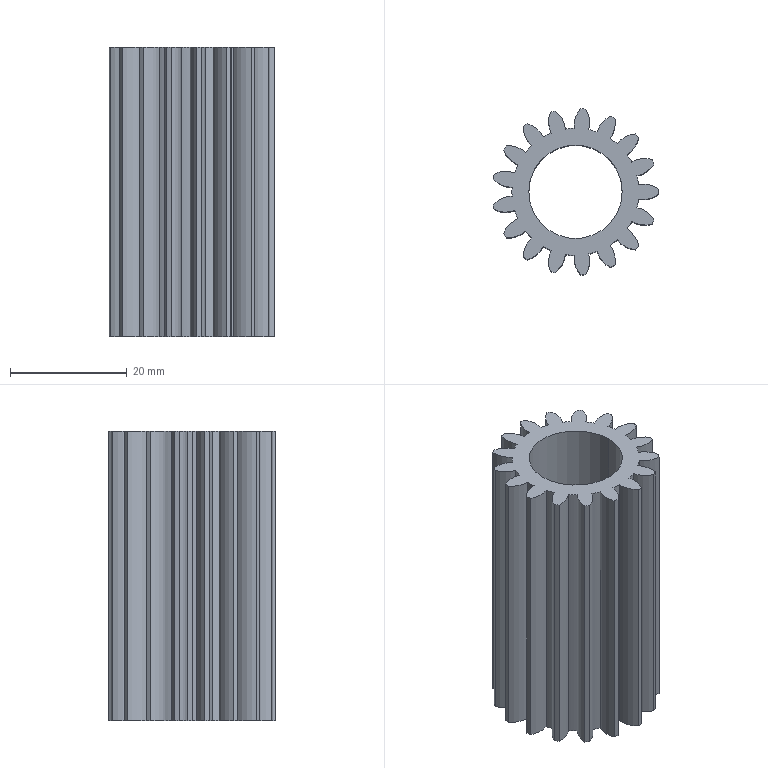Part | SolidWorks | features CirPattern 1, Extrusion 1, ICE 1 | 1 solid | 78 faces | box 28.328 x 28.443 x 49.5 mm | volume 14667 mm3 | cylinder 76 | plane 2 | commonest cylinder face diameters 8.722 x38 21.75 x18 28.5 x18 16 x2